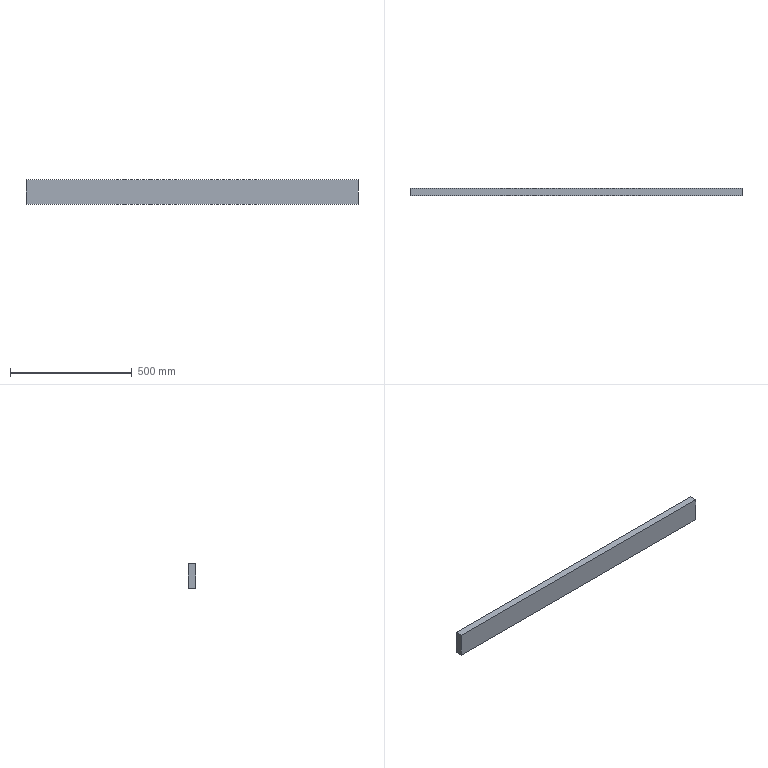Part | SolidWorks | features Extrusion 1 | 1 solid | 6 faces | box 1364 x 30 x 100 mm | volume 4092000 mm3 | plane 6
STEP:
#1=CARTESIAN_POINT('',(682.,0.,50.));
#2=VERTEX_POINT('',#1);
#3=CARTESIAN_POINT('',(682.,0.,-50.));
#4=VERTEX_POINT('',#3);
#5=CARTESIAN_POINT('',(682.,0.,50.));
#6=DIRECTION('',(0.,0.,-1.));
#7=VECTOR('',#6,1000.);
#8=LINE('',#5,#7);
#9=EDGE_CURVE('',#2,#4,#8,.T.);
#10=ORIENTED_EDGE('',*,*,#9,.T.);
#11=CARTESIAN_POINT('',(682.,30.,-50.));
#12=VERTEX_POINT('',#11);
#13=CARTESIAN_POINT('',(682.,30.,-50.));
#14=DIRECTION('',(0.,-1.,0.));
#15=VECTOR('',#14,1000.);
#16=LINE('',#13,#15);
#17=EDGE_CURVE('',#12,#4,#16,.T.);
#18=ORIENTED_EDGE('',*,*,#17,.F.);
#19=CARTESIAN_POINT('',(682.,30.,50.));
#20=VERTEX_POINT('',#19);
#21=CARTESIAN_POINT('',(682.,30.,50.));
#22=DIRECTION('',(0.,0.,-1.));
#23=VECTOR('',#22,1000.);
#24=LINE('',#21,#23);
#25=EDGE_CURVE('',#20,#12,#24,.T.);
#26=ORIENTED_EDGE('',*,*,#25,.F.);
#27=CARTESIAN_POINT('',(682.,30.,50.));
#28=DIRECTION('',(0.,-1.,0.));
#29=VECTOR('',#28,1000.);
#30=LINE('',#27,#29);
#31=EDGE_CURVE('',#20,#2,#30,.T.);
#32=ORIENTED_EDGE('',*,*,#31,.T.);
#33=EDGE_LOOP('',(#10,#18,#26,#32));
#34=FACE_OUTER_BOUND('',#33,.T.);
#35=CARTESIAN_POINT('',(682.,30.,50.));
#36=DIRECTION('',(-1.,0.,0.));
#37=DIRECTION('',(0.,0.,1.));
#38=AXIS2_PLACEMENT_3D('',#35,#36,#37);
#39=PLANE('',#38);
#40=ADVANCED_FACE('',(#34),#39,.F.);
#41=CARTESIAN_POINT('',(-682.,0.,-50.));
#42=VERTEX_POINT('',#41);
#43=CARTESIAN_POINT('',(-682.,0.,-50.));
#44=DIRECTION('',(-1.,0.,0.));
#45=VECTOR('',#44,1000.);
#46=LINE('',#43,#45);
#47=EDGE_CURVE('',#4,#42,#46,.T.);
#48=ORIENTED_EDGE('',*,*,#47,.T.);
#49=CARTESIAN_POINT('',(-682.,30.,-50.));
#50=VERTEX_POINT('',#49);
#51=CARTESIAN_POINT('',(-682.,30.,-50.));
#52=DIRECTION('',(0.,-1.,0.));
#53=VECTOR('',#52,1000.);
#54=LINE('',#51,#53);
#55=EDGE_CURVE('',#50,#42,#54,.T.);
#56=ORIENTED_EDGE('',*,*,#55,.F.);
#57=CARTESIAN_POINT('',(-682.,30.,-50.));
#58=DIRECTION('',(-1.,0.,0.));
#59=VECTOR('',#58,1000.);
#60=LINE('',#57,#59);
#61=EDGE_CURVE('',#12,#50,#60,.T.);
#62=ORIENTED_EDGE('',*,*,#61,.F.);
#63=ORIENTED_EDGE('',*,*,#17,.T.);
#64=EDGE_LOOP('',(#48,#56,#62,#63));
#65=FACE_OUTER_BOUND('',#64,.T.);
#66=CARTESIAN_POINT('',(-682.,30.,-50.));
#67=DIRECTION('',(0.,0.,1.));
#68=DIRECTION('',(1.,0.,0.));
#69=AXIS2_PLACEMENT_3D('',#66,#67,#68);
#70=PLANE('',#69);
#71=ADVANCED_FACE('',(#65),#70,.F.);
#72=CARTESIAN_POINT('',(-682.,0.,50.));
#73=VERTEX_POINT('',#72);
#74=CARTESIAN_POINT('',(-682.,0.,50.));
#75=DIRECTION('',(0.,0.,1.));
#76=VECTOR('',#75,1000.);
#77=LINE('',#74,#76);
#78=EDGE_CURVE('',#42,#73,#77,.T.);
#79=ORIENTED_EDGE('',*,*,#78,.T.);
#80=CARTESIAN_POINT('',(-682.,30.,50.));
#81=VERTEX_POINT('',#80);
#82=CARTESIAN_POINT('',(-682.,30.,50.));
#83=DIRECTION('',(0.,-1.,0.));
#84=VECTOR('',#83,1000.);
#85=LINE('',#82,#84);
#86=EDGE_CURVE('',#81,#73,#85,.T.);
#87=ORIENTED_EDGE('',*,*,#86,.F.);
#88=CARTESIAN_POINT('',(-682.,30.,50.));
#89=DIRECTION('',(0.,0.,1.));
#90=VECTOR('',#89,1000.);
#91=LINE('',#88,#90);
#92=EDGE_CURVE('',#50,#81,#91,.T.);
#93=ORIENTED_EDGE('',*,*,#92,.F.);
#94=ORIENTED_EDGE('',*,*,#55,.T.);
#95=EDGE_LOOP('',(#79,#87,#93,#94));
#96=FACE_OUTER_BOUND('',#95,.T.);
#97=CARTESIAN_POINT('',(-682.,30.,50.));
#98=DIRECTION('',(1.,0.,0.));
#99=DIRECTION('',(0.,0.,-1.));
#100=AXIS2_PLACEMENT_3D('',#97,#98,#99);
#101=PLANE('',#100);
#102=ADVANCED_FACE('',(#96),#101,.F.);
#103=CARTESIAN_POINT('',(-682.,0.,50.));
#104=DIRECTION('',(1.,0.,0.));
#105=VECTOR('',#104,1000.);
#106=LINE('',#103,#105);
#107=EDGE_CURVE('',#73,#2,#106,.T.);
#108=ORIENTED_EDGE('',*,*,#107,.T.);
#109=ORIENTED_EDGE('',*,*,#31,.F.);
#110=CARTESIAN_POINT('',(-682.,30.,50.));
#111=DIRECTION('',(1.,0.,0.));
#112=VECTOR('',#111,1000.);
#113=LINE('',#110,#112);
#114=EDGE_CURVE('',#81,#20,#113,.T.);
#115=ORIENTED_EDGE('',*,*,#114,.F.);
#116=ORIENTED_EDGE('',*,*,#86,.T.);
#117=EDGE_LOOP('',(#108,#109,#115,#116));
#118=FACE_OUTER_BOUND('',#117,.T.);
#119=CARTESIAN_POINT('',(-682.,30.,50.));
#120=DIRECTION('',(0.,0.,-1.));
#121=DIRECTION('',(-1.,0.,0.));
#122=AXIS2_PLACEMENT_3D('',#119,#120,#121);
#123=PLANE('',#122);
#124=ADVANCED_FACE('',(#118),#123,.F.);
#125=ORIENTED_EDGE('',*,*,#25,.T.);
#126=ORIENTED_EDGE('',*,*,#61,.T.);
#127=ORIENTED_EDGE('',*,*,#92,.T.);
#128=ORIENTED_EDGE('',*,*,#114,.T.);
#129=EDGE_LOOP('',(#125,#126,#127,#128));
#130=FACE_OUTER_BOUND('',#129,.T.);
#131=CARTESIAN_POINT('',(0.,30.,0.));
#132=DIRECTION('',(0.,-1.,0.));
#133=DIRECTION('',(0.,0.,-1.));
#134=AXIS2_PLACEMENT_3D('',#131,#132,#133);
#135=PLANE('',#134);
#136=ADVANCED_FACE('',(#130),#135,.F.);
#137=ORIENTED_EDGE('',*,*,#9,.F.);
#138=ORIENTED_EDGE('',*,*,#107,.F.);
#139=ORIENTED_EDGE('',*,*,#78,.F.);
#140=ORIENTED_EDGE('',*,*,#47,.F.);
#141=EDGE_LOOP('',(#137,#138,#139,#140));
#142=FACE_OUTER_BOUND('',#141,.T.);
#143=CARTESIAN_POINT('',(0.,0.,0.));
#144=DIRECTION('',(0.,-1.,0.));
#145=DIRECTION('',(0.,0.,-1.));
#146=AXIS2_PLACEMENT_3D('',#143,#144,#145);
#147=PLANE('',#146);
#148=ADVANCED_FACE('',(#142),#147,.T.);
#149=CLOSED_SHELL('',(#40,#71,#102,#124,#136,#148));
#150=MANIFOLD_SOLID_BREP('',#149);
#151=CARTESIAN_POINT('',(0.,0.,0.));
#152=DIRECTION('',(0.,0.,1.));
#153=DIRECTION('',(1.,0.,0.));
#154=AXIS2_PLACEMENT_3D('',#151,#152,#153);
#155=(LENGTH_UNIT()NAMED_UNIT(*)SI_UNIT(.MILLI.,.METRE.));
#156=UNCERTAINTY_MEASURE_WITH_UNIT(LENGTH_MEASURE(0.00001),#155,'','');
#157=(NAMED_UNIT(*)PLANE_ANGLE_UNIT()SI_UNIT($,.RADIAN.));
#158=(NAMED_UNIT(*)SI_UNIT($,.STERADIAN.)SOLID_ANGLE_UNIT());
#159=(GEOMETRIC_REPRESENTATION_CONTEXT(3)GLOBAL_UNCERTAINTY_ASSIGNED_CONTEXT((#156))GLOBAL_UNIT_ASSIGNED_CONTEXT((#155,#157,#158))REPRESENTATION_CONTEXT('',''));
#160=ADVANCED_BREP_SHAPE_REPRESENTATION('',(#150,#154),#159);